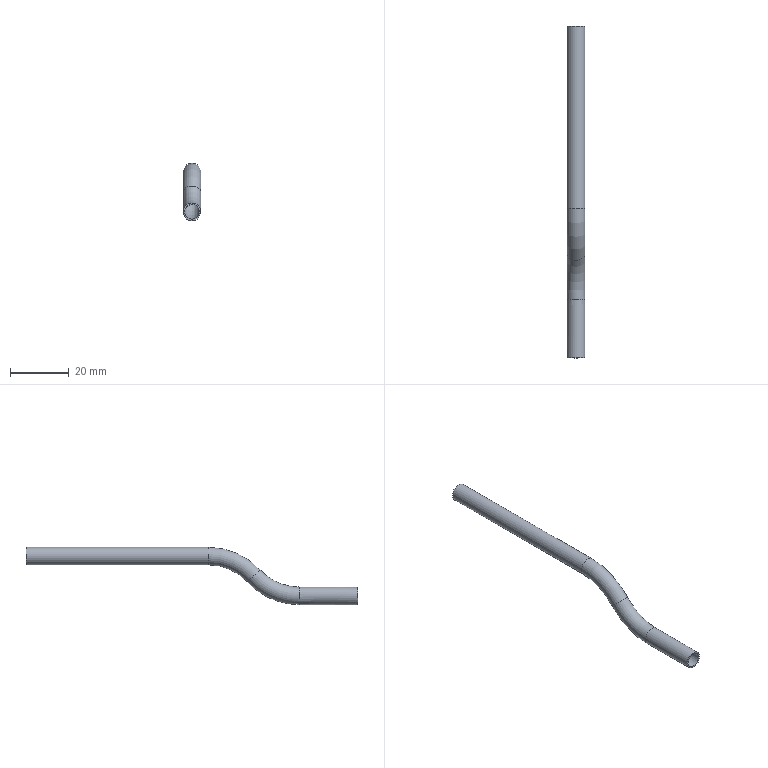Part | STEP file | 1-75.8 | 1 solid | 10 faces | box 6 x 112.85 x 19.5 mm | volume 1008 mm3 | cylinder 4 | torus 4 | plane 2 | commonest cylinder face diameters 5 x2 6 x2
STEP:
#1=CARTESIAN_POINT('',(0.,0.,0.));
#2=DIRECTION('',(0.,0.,1.));
#3=DIRECTION('',(1.,0.,0.));
#4=AXIS2_PLACEMENT_3D('',#1,#2,#3);
#5=CARTESIAN_POINT('',(3.,0.,0.));
#6=VERTEX_POINT('',#5);
#7=CARTESIAN_POINT('',(0.,0.,0.));
#8=DIRECTION('',(0.,-1.,0.));
#9=DIRECTION('',(1.,0.,0.));
#10=AXIS2_PLACEMENT_3D('',#7,#8,#9);
#11=CIRCLE('',#10,3.);
#12=CARTESIAN_POINT('',(0.,0.,0.));
#13=DIRECTION('',(0.,1.,0.));
#14=DIRECTION('',(1.,0.,0.));
#15=AXIS2_PLACEMENT_3D('',#12,#13,#14);
#16=CYLINDRICAL_SURFACE('',#15,3.);
#17=CARTESIAN_POINT('',(6.283,0.));
#18=DIRECTION('',(-1.,0.));
#19=VECTOR('',#18,1.);
#20=LINE('',#17,#19);
#21=(GEOMETRIC_REPRESENTATION_CONTEXT(2)PARAMETRIC_REPRESENTATION_CONTEXT()REPRESENTATION_CONTEXT('',''));
#22=DEFINITIONAL_REPRESENTATION('',(#20),#21);
#23=PCURVE('',#16,#22);
#24=CARTESIAN_POINT('',(0.,0.,0.));
#25=DIRECTION('',(0.,-1.,0.));
#26=DIRECTION('',(0.,0.,-1.));
#27=AXIS2_PLACEMENT_3D('',#24,#25,#26);
#28=PLANE('',#27);
#29=CARTESIAN_POINT('',(0.,0.));
#30=DIRECTION('',(0.,1.));
#31=AXIS2_PLACEMENT_2D('',#29,#30);
#32=CIRCLE('',#31,3.);
#33=(GEOMETRIC_REPRESENTATION_CONTEXT(2)PARAMETRIC_REPRESENTATION_CONTEXT()REPRESENTATION_CONTEXT('',''));
#34=DEFINITIONAL_REPRESENTATION('',(#32),#33);
#35=PCURVE('',#28,#34);
#36=SURFACE_CURVE('',#11,(#23,#35),.PCURVE_S1.);
#37=EDGE_CURVE('',#6,#6,#36,.T.);
#38=ORIENTED_EDGE('',*,*,#37,.F.);
#39=CARTESIAN_POINT('',(3.,20.,0.));
#40=VERTEX_POINT('',#39);
#41=CARTESIAN_POINT('',(3.,0.,0.));
#42=DIRECTION('',(0.,1.,0.));
#43=VECTOR('',#42,1.);
#44=LINE('',#41,#43);
#45=CARTESIAN_POINT('',(6.283,0.));
#46=DIRECTION('',(0.,1.));
#47=VECTOR('',#46,1.);
#48=LINE('',#45,#47);
#49=(GEOMETRIC_REPRESENTATION_CONTEXT(2)PARAMETRIC_REPRESENTATION_CONTEXT()REPRESENTATION_CONTEXT('',''));
#50=DEFINITIONAL_REPRESENTATION('',(#48),#49);
#51=PCURVE('',#16,#50);
#52=CARTESIAN_POINT('',(0.,0.));
#53=DIRECTION('',(0.,1.));
#54=VECTOR('',#53,1.);
#55=LINE('',#52,#54);
#56=(GEOMETRIC_REPRESENTATION_CONTEXT(2)PARAMETRIC_REPRESENTATION_CONTEXT()REPRESENTATION_CONTEXT('',''));
#57=DEFINITIONAL_REPRESENTATION('',(#55),#56);
#58=PCURVE('',#16,#57);
#59=SEAM_CURVE('',#44,(#51,#58),.PCURVE_S1.);
#60=EDGE_CURVE('',#6,#40,#59,.T.);
#61=ORIENTED_EDGE('',*,*,#60,.T.);
#62=CARTESIAN_POINT('',(0.,20.,-3.));
#63=VERTEX_POINT('',#62);
#64=CARTESIAN_POINT('',(0.,20.,0.));
#65=DIRECTION('',(0.,1.,0.));
#66=DIRECTION('',(0.,0.,-1.));
#67=AXIS2_PLACEMENT_3D('',#64,#65,#66);
#68=CIRCLE('',#67,3.);
#69=CARTESIAN_POINT('',(1.571,20.));
#70=DIRECTION('',(1.,0.));
#71=VECTOR('',#70,1.);
#72=LINE('',#69,#71);
#73=(GEOMETRIC_REPRESENTATION_CONTEXT(2)PARAMETRIC_REPRESENTATION_CONTEXT()REPRESENTATION_CONTEXT('',''));
#74=DEFINITIONAL_REPRESENTATION('',(#72),#73);
#75=PCURVE('',#16,#74);
#76=CARTESIAN_POINT('',(0.,20.,21.));
#77=DIRECTION('',(-1.,0.,0.));
#78=DIRECTION('',(0.,0.,-1.));
#79=AXIS2_PLACEMENT_3D('',#76,#77,#78);
#80=TOROIDAL_SURFACE('',#79,21.,3.);
#81=CARTESIAN_POINT('',(6.283,0.));
#82=DIRECTION('',(0.,1.));
#83=VECTOR('',#82,1.);
#84=LINE('',#81,#83);
#85=(GEOMETRIC_REPRESENTATION_CONTEXT(2)PARAMETRIC_REPRESENTATION_CONTEXT()REPRESENTATION_CONTEXT('',''));
#86=DEFINITIONAL_REPRESENTATION('',(#84),#85);
#87=PCURVE('',#80,#86);
#88=SURFACE_CURVE('',#68,(#75,#87),.PCURVE_S1.);
#89=EDGE_CURVE('',#63,#40,#88,.T.);
#90=ORIENTED_EDGE('',*,*,#89,.F.);
#91=CARTESIAN_POINT('',(0.,20.,0.));
#92=DIRECTION('',(0.,1.,0.));
#93=DIRECTION('',(1.,0.,0.));
#94=AXIS2_PLACEMENT_3D('',#91,#92,#93);
#95=CIRCLE('',#94,3.);
#96=CARTESIAN_POINT('',(0.,20.));
#97=DIRECTION('',(1.,0.));
#98=VECTOR('',#97,1.);
#99=LINE('',#96,#98);
#100=(GEOMETRIC_REPRESENTATION_CONTEXT(2)PARAMETRIC_REPRESENTATION_CONTEXT()REPRESENTATION_CONTEXT('',''));
#101=DEFINITIONAL_REPRESENTATION('',(#99),#100);
#102=PCURVE('',#16,#101);
#103=CARTESIAN_POINT('',(6.283,4.712));
#104=DIRECTION('',(0.,1.));
#105=VECTOR('',#104,1.);
#106=LINE('',#103,#105);
#107=(GEOMETRIC_REPRESENTATION_CONTEXT(2)PARAMETRIC_REPRESENTATION_CONTEXT()REPRESENTATION_CONTEXT('',''));
#108=DEFINITIONAL_REPRESENTATION('',(#106),#107);
#109=PCURVE('',#80,#108);
#110=SURFACE_CURVE('',#95,(#102,#109),.PCURVE_S1.);
#111=EDGE_CURVE('',#40,#63,#110,.T.);
#112=ORIENTED_EDGE('',*,*,#111,.F.);
#113=ORIENTED_EDGE('',*,*,#60,.F.);
#114=EDGE_LOOP('',(#38,#61,#90,#112,#113));
#115=FACE_BOUND('',#114,.T.);
#116=ADVANCED_FACE('',(#115),#16,.T.);
#117=ORIENTED_EDGE('',*,*,#89,.T.);
#118=ORIENTED_EDGE('',*,*,#111,.T.);
#119=CARTESIAN_POINT('',(0.,37.629,4.714));
#120=VERTEX_POINT('',#119);
#121=CARTESIAN_POINT('',(0.,20.,21.));
#122=DIRECTION('',(1.,0.,0.));
#123=DIRECTION('',(0.,0.,-1.));
#124=AXIS2_PLACEMENT_3D('',#121,#122,#123);
#125=CIRCLE('',#124,24.);
#126=CARTESIAN_POINT('',(6.283,6.283));
#127=DIRECTION('',(-1.,0.));
#128=VECTOR('',#127,1.);
#129=LINE('',#126,#128);
#130=(GEOMETRIC_REPRESENTATION_CONTEXT(2)PARAMETRIC_REPRESENTATION_CONTEXT()REPRESENTATION_CONTEXT('',''));
#131=DEFINITIONAL_REPRESENTATION('',(#129),#130);
#132=PCURVE('',#80,#131);
#133=CARTESIAN_POINT('',(6.283,0.));
#134=DIRECTION('',(-1.,0.));
#135=VECTOR('',#134,1.);
#136=LINE('',#133,#135);
#137=(GEOMETRIC_REPRESENTATION_CONTEXT(2)PARAMETRIC_REPRESENTATION_CONTEXT()REPRESENTATION_CONTEXT('',''));
#138=DEFINITIONAL_REPRESENTATION('',(#136),#137);
#139=PCURVE('',#80,#138);
#140=SEAM_CURVE('',#125,(#132,#139),.PCURVE_S1.);
#141=EDGE_CURVE('',#63,#120,#140,.T.);
#142=ORIENTED_EDGE('',*,*,#141,.T.);
#143=CARTESIAN_POINT('',(-3.,35.425,6.75));
#144=VERTEX_POINT('',#143);
#145=CARTESIAN_POINT('',(0.,35.425,6.75));
#146=DIRECTION('',(0.,-0.6786,-0.7345));
#147=DIRECTION('',(0.,0.7345,-0.6786));
#148=AXIS2_PLACEMENT_3D('',#145,#146,#147);
#149=CIRCLE('',#148,3.);
#150=CARTESIAN_POINT('',(5.458,6.283));
#151=DIRECTION('',(0.,-1.));
#152=VECTOR('',#151,1.);
#153=LINE('',#150,#152);
#154=(GEOMETRIC_REPRESENTATION_CONTEXT(2)PARAMETRIC_REPRESENTATION_CONTEXT()REPRESENTATION_CONTEXT('',''));
#155=DEFINITIONAL_REPRESENTATION('',(#153),#154);
#156=PCURVE('',#80,#155);
#157=CARTESIAN_POINT('',(0.,50.85,-7.5));
#158=DIRECTION('',(1.,0.,0.));
#159=DIRECTION('',(0.,-0.7345,0.6786));
#160=AXIS2_PLACEMENT_3D('',#157,#158,#159);
#161=TOROIDAL_SURFACE('',#160,21.,3.);
#162=CARTESIAN_POINT('',(6.283,3.142));
#163=DIRECTION('',(0.,-1.));
#164=VECTOR('',#163,1.);
#165=LINE('',#162,#164);
#166=(GEOMETRIC_REPRESENTATION_CONTEXT(2)PARAMETRIC_REPRESENTATION_CONTEXT()REPRESENTATION_CONTEXT('',''));
#167=DEFINITIONAL_REPRESENTATION('',(#165),#166);
#168=PCURVE('',#161,#167);
#169=SURFACE_CURVE('',#149,(#156,#168),.PCURVE_S1.);
#170=EDGE_CURVE('',#120,#144,#169,.T.);
#171=ORIENTED_EDGE('',*,*,#170,.T.);
#172=CARTESIAN_POINT('',(0.,35.425,6.75));
#173=DIRECTION('',(0.,-0.6786,-0.7345));
#174=DIRECTION('',(-1.,0.,0.));
#175=AXIS2_PLACEMENT_3D('',#172,#173,#174);
#176=CIRCLE('',#175,3.);
#177=CARTESIAN_POINT('',(5.458,1.571));
#178=DIRECTION('',(0.,-1.));
#179=VECTOR('',#178,1.);
#180=LINE('',#177,#179);
#181=(GEOMETRIC_REPRESENTATION_CONTEXT(2)PARAMETRIC_REPRESENTATION_CONTEXT()REPRESENTATION_CONTEXT('',''));
#182=DEFINITIONAL_REPRESENTATION('',(#180),#181);
#183=PCURVE('',#80,#182);
#184=CARTESIAN_POINT('',(6.283,4.712));
#185=DIRECTION('',(0.,-1.));
#186=VECTOR('',#185,1.);
#187=LINE('',#184,#186);
#188=(GEOMETRIC_REPRESENTATION_CONTEXT(2)PARAMETRIC_REPRESENTATION_CONTEXT()REPRESENTATION_CONTEXT('',''));
#189=DEFINITIONAL_REPRESENTATION('',(#187),#188);
#190=PCURVE('',#161,#189);
#191=SURFACE_CURVE('',#176,(#183,#190),.PCURVE_S1.);
#192=EDGE_CURVE('',#144,#120,#191,.T.);
#193=ORIENTED_EDGE('',*,*,#192,.T.);
#194=ORIENTED_EDGE('',*,*,#141,.F.);
#195=EDGE_LOOP('',(#117,#118,#142,#171,#193,#194));
#196=FACE_BOUND('',#195,.T.);
#197=ADVANCED_FACE('',(#196),#80,.T.);
#198=ORIENTED_EDGE('',*,*,#170,.F.);
#199=ORIENTED_EDGE('',*,*,#192,.F.);
#200=CARTESIAN_POINT('',(-3.,50.85,13.5));
#201=VERTEX_POINT('',#200);
#202=CARTESIAN_POINT('',(-3.,50.85,-7.5));
#203=DIRECTION('',(-1.,0.,0.));
#204=DIRECTION('',(0.,-0.7345,0.6786));
#205=AXIS2_PLACEMENT_3D('',#202,#203,#204);
#206=CIRCLE('',#205,21.);
#207=CARTESIAN_POINT('',(6.283,4.712));
#208=DIRECTION('',(-1.,0.));
#209=VECTOR('',#208,1.);
#210=LINE('',#207,#209);
#211=(GEOMETRIC_REPRESENTATION_CONTEXT(2)PARAMETRIC_REPRESENTATION_CONTEXT()REPRESENTATION_CONTEXT('',''));
#212=DEFINITIONAL_REPRESENTATION('',(#210),#211);
#213=PCURVE('',#161,#212);
#214=CARTESIAN_POINT('',(6.283,-1.571));
#215=DIRECTION('',(-1.,0.));
#216=VECTOR('',#215,1.);
#217=LINE('',#214,#216);
#218=(GEOMETRIC_REPRESENTATION_CONTEXT(2)PARAMETRIC_REPRESENTATION_CONTEXT()REPRESENTATION_CONTEXT('',''));
#219=DEFINITIONAL_REPRESENTATION('',(#217),#218);
#220=PCURVE('',#161,#219);
#221=SEAM_CURVE('',#206,(#213,#220),.PCURVE_S1.);
#222=EDGE_CURVE('',#144,#201,#221,.T.);
#223=ORIENTED_EDGE('',*,*,#222,.T.);
#224=CARTESIAN_POINT('',(3.,50.85,13.5));
#225=VERTEX_POINT('',#224);
#226=CARTESIAN_POINT('',(0.,50.85,13.5));
#227=DIRECTION('',(0.,-1.,0.));
#228=DIRECTION('',(-1.,0.,0.));
#229=AXIS2_PLACEMENT_3D('',#226,#227,#228);
#230=CIRCLE('',#229,3.);
#231=CARTESIAN_POINT('',(5.458,4.712));
#232=DIRECTION('',(0.,-1.));
#233=VECTOR('',#232,1.);
#234=LINE('',#231,#233);
#235=(GEOMETRIC_REPRESENTATION_CONTEXT(2)PARAMETRIC_REPRESENTATION_CONTEXT()REPRESENTATION_CONTEXT('',''));
#236=DEFINITIONAL_REPRESENTATION('',(#234),#235);
#237=PCURVE('',#161,#236);
#238=CARTESIAN_POINT('',(0.,50.85,13.5));
#239=DIRECTION('',(0.,1.,0.));
#240=DIRECTION('',(1.,0.,0.));
#241=AXIS2_PLACEMENT_3D('',#238,#239,#240);
#242=CYLINDRICAL_SURFACE('',#241,3.);
#243=CARTESIAN_POINT('',(3.142,0.));
#244=DIRECTION('',(-1.,0.));
#245=VECTOR('',#244,1.);
#246=LINE('',#243,#245);
#247=(GEOMETRIC_REPRESENTATION_CONTEXT(2)PARAMETRIC_REPRESENTATION_CONTEXT()REPRESENTATION_CONTEXT('',''));
#248=DEFINITIONAL_REPRESENTATION('',(#246),#247);
#249=PCURVE('',#242,#248);
#250=SURFACE_CURVE('',#230,(#237,#249),.PCURVE_S1.);
#251=EDGE_CURVE('',#201,#225,#250,.T.);
#252=ORIENTED_EDGE('',*,*,#251,.T.);
#253=CARTESIAN_POINT('',(0.,50.85,13.5));
#254=DIRECTION('',(0.,-1.,0.));
#255=DIRECTION('',(1.,0.,0.));
#256=AXIS2_PLACEMENT_3D('',#253,#254,#255);
#257=CIRCLE('',#256,3.);
#258=CARTESIAN_POINT('',(5.458,1.571));
#259=DIRECTION('',(0.,-1.));
#260=VECTOR('',#259,1.);
#261=LINE('',#258,#260);
#262=(GEOMETRIC_REPRESENTATION_CONTEXT(2)PARAMETRIC_REPRESENTATION_CONTEXT()REPRESENTATION_CONTEXT('',''));
#263=DEFINITIONAL_REPRESENTATION('',(#261),#262);
#264=PCURVE('',#161,#263);
#265=CARTESIAN_POINT('',(6.283,0.));
#266=DIRECTION('',(-1.,0.));
#267=VECTOR('',#266,1.);
#268=LINE('',#265,#267);
#269=(GEOMETRIC_REPRESENTATION_CONTEXT(2)PARAMETRIC_REPRESENTATION_CONTEXT()REPRESENTATION_CONTEXT('',''));
#270=DEFINITIONAL_REPRESENTATION('',(#268),#269);
#271=PCURVE('',#242,#270);
#272=SURFACE_CURVE('',#257,(#264,#271),.PCURVE_S1.);
#273=EDGE_CURVE('',#225,#201,#272,.T.);
#274=ORIENTED_EDGE('',*,*,#273,.T.);
#275=ORIENTED_EDGE('',*,*,#222,.F.);
#276=EDGE_LOOP('',(#198,#199,#223,#252,#274,#275));
#277=FACE_BOUND('',#276,.T.);
#278=ADVANCED_FACE('',(#277),#161,.T.);
#279=ORIENTED_EDGE('',*,*,#251,.F.);
#280=ORIENTED_EDGE('',*,*,#273,.F.);
#281=CARTESIAN_POINT('',(3.,112.85,13.5));
#282=VERTEX_POINT('',#281);
#283=CARTESIAN_POINT('',(3.,50.85,13.5));
#284=DIRECTION('',(0.,1.,0.));
#285=VECTOR('',#284,1.);
#286=LINE('',#283,#285);
#287=CARTESIAN_POINT('',(6.283,0.));
#288=DIRECTION('',(0.,1.));
#289=VECTOR('',#288,1.);
#290=LINE('',#287,#289);
#291=(GEOMETRIC_REPRESENTATION_CONTEXT(2)PARAMETRIC_REPRESENTATION_CONTEXT()REPRESENTATION_CONTEXT('',''));
#292=DEFINITIONAL_REPRESENTATION('',(#290),#291);
#293=PCURVE('',#242,#292);
#294=CARTESIAN_POINT('',(0.,0.));
#295=DIRECTION('',(0.,1.));
#296=VECTOR('',#295,1.);
#297=LINE('',#294,#296);
#298=(GEOMETRIC_REPRESENTATION_CONTEXT(2)PARAMETRIC_REPRESENTATION_CONTEXT()REPRESENTATION_CONTEXT('',''));
#299=DEFINITIONAL_REPRESENTATION('',(#297),#298);
#300=PCURVE('',#242,#299);
#301=SEAM_CURVE('',#286,(#293,#300),.PCURVE_S1.);
#302=EDGE_CURVE('',#225,#282,#301,.T.);
#303=ORIENTED_EDGE('',*,*,#302,.T.);
#304=CARTESIAN_POINT('',(0.,112.85,13.5));
#305=DIRECTION('',(0.,1.,0.));
#306=DIRECTION('',(1.,0.,0.));
#307=AXIS2_PLACEMENT_3D('',#304,#305,#306);
#308=CIRCLE('',#307,3.);
#309=CARTESIAN_POINT('',(0.,62.));
#310=DIRECTION('',(1.,0.));
#311=VECTOR('',#310,1.);
#312=LINE('',#309,#311);
#313=(GEOMETRIC_REPRESENTATION_CONTEXT(2)PARAMETRIC_REPRESENTATION_CONTEXT()REPRESENTATION_CONTEXT('',''));
#314=DEFINITIONAL_REPRESENTATION('',(#312),#313);
#315=PCURVE('',#242,#314);
#316=CARTESIAN_POINT('',(0.,112.85,13.5));
#317=DIRECTION('',(0.,1.,0.));
#318=DIRECTION('',(0.,0.,1.));
#319=AXIS2_PLACEMENT_3D('',#316,#317,#318);
#320=PLANE('',#319);
#321=CARTESIAN_POINT('',(0.,0.));
#322=DIRECTION('',(0.,1.));
#323=AXIS2_PLACEMENT_2D('',#321,#322);
#324=CIRCLE('',#323,3.);
#325=(GEOMETRIC_REPRESENTATION_CONTEXT(2)PARAMETRIC_REPRESENTATION_CONTEXT()REPRESENTATION_CONTEXT('',''));
#326=DEFINITIONAL_REPRESENTATION('',(#324),#325);
#327=PCURVE('',#320,#326);
#328=SURFACE_CURVE('',#308,(#315,#327),.PCURVE_S1.);
#329=EDGE_CURVE('',#282,#282,#328,.T.);
#330=ORIENTED_EDGE('',*,*,#329,.F.);
#331=ORIENTED_EDGE('',*,*,#302,.F.);
#332=EDGE_LOOP('',(#279,#280,#303,#330,#331));
#333=FACE_BOUND('',#332,.T.);
#334=ADVANCED_FACE('',(#333),#242,.T.);
#335=ORIENTED_EDGE('',*,*,#37,.T.);
#336=EDGE_LOOP('',(#335));
#337=FACE_BOUND('',#336,.T.);
#338=CARTESIAN_POINT('',(2.5,0.,0.));
#339=VERTEX_POINT('',#338);
#340=CARTESIAN_POINT('',(0.,0.,0.));
#341=DIRECTION('',(0.,-1.,0.));
#342=DIRECTION('',(1.,0.,0.));
#343=AXIS2_PLACEMENT_3D('',#340,#341,#342);
#344=CIRCLE('',#343,2.5);
#345=CARTESIAN_POINT('',(0.,0.));
#346=DIRECTION('',(0.,1.));
#347=AXIS2_PLACEMENT_2D('',#345,#346);
#348=CIRCLE('',#347,2.5);
#349=(GEOMETRIC_REPRESENTATION_CONTEXT(2)PARAMETRIC_REPRESENTATION_CONTEXT()REPRESENTATION_CONTEXT('',''));
#350=DEFINITIONAL_REPRESENTATION('',(#348),#349);
#351=PCURVE('',#28,#350);
#352=CARTESIAN_POINT('',(0.,0.,0.));
#353=DIRECTION('',(0.,1.,0.));
#354=DIRECTION('',(1.,0.,0.));
#355=AXIS2_PLACEMENT_3D('',#352,#353,#354);
#356=CYLINDRICAL_SURFACE('',#355,2.5);
#357=CARTESIAN_POINT('',(6.283,0.));
#358=DIRECTION('',(-1.,0.));
#359=VECTOR('',#358,1.);
#360=LINE('',#357,#359);
#361=(GEOMETRIC_REPRESENTATION_CONTEXT(2)PARAMETRIC_REPRESENTATION_CONTEXT()REPRESENTATION_CONTEXT('',''));
#362=DEFINITIONAL_REPRESENTATION('',(#360),#361);
#363=PCURVE('',#356,#362);
#364=SURFACE_CURVE('',#344,(#351,#363),.PCURVE_S1.);
#365=EDGE_CURVE('',#339,#339,#364,.T.);
#366=ORIENTED_EDGE('',*,*,#365,.F.);
#367=EDGE_LOOP('',(#366));
#368=FACE_BOUND('',#367,.T.);
#369=ADVANCED_FACE('',(#337,#368),#28,.T.);
#370=ORIENTED_EDGE('',*,*,#329,.T.);
#371=EDGE_LOOP('',(#370));
#372=FACE_BOUND('',#371,.T.);
#373=CARTESIAN_POINT('',(2.5,112.85,13.5));
#374=VERTEX_POINT('',#373);
#375=CARTESIAN_POINT('',(0.,112.85,13.5));
#376=DIRECTION('',(0.,1.,0.));
#377=DIRECTION('',(1.,0.,0.));
#378=AXIS2_PLACEMENT_3D('',#375,#376,#377);
#379=CIRCLE('',#378,2.5);
#380=CARTESIAN_POINT('',(0.,0.));
#381=DIRECTION('',(0.,1.));
#382=AXIS2_PLACEMENT_2D('',#380,#381);
#383=CIRCLE('',#382,2.5);
#384=(GEOMETRIC_REPRESENTATION_CONTEXT(2)PARAMETRIC_REPRESENTATION_CONTEXT()REPRESENTATION_CONTEXT('',''));
#385=DEFINITIONAL_REPRESENTATION('',(#383),#384);
#386=PCURVE('',#320,#385);
#387=CARTESIAN_POINT('',(0.,50.85,13.5));
#388=DIRECTION('',(0.,1.,0.));
#389=DIRECTION('',(1.,0.,0.));
#390=AXIS2_PLACEMENT_3D('',#387,#388,#389);
#391=CYLINDRICAL_SURFACE('',#390,2.5);
#392=CARTESIAN_POINT('',(0.,62.));
#393=DIRECTION('',(1.,0.));
#394=VECTOR('',#393,1.);
#395=LINE('',#392,#394);
#396=(GEOMETRIC_REPRESENTATION_CONTEXT(2)PARAMETRIC_REPRESENTATION_CONTEXT()REPRESENTATION_CONTEXT('',''));
#397=DEFINITIONAL_REPRESENTATION('',(#395),#396);
#398=PCURVE('',#391,#397);
#399=SURFACE_CURVE('',#379,(#386,#398),.PCURVE_S1.);
#400=EDGE_CURVE('',#374,#374,#399,.T.);
#401=ORIENTED_EDGE('',*,*,#400,.F.);
#402=EDGE_LOOP('',(#401));
#403=FACE_BOUND('',#402,.T.);
#404=ADVANCED_FACE('',(#372,#403),#320,.T.);
#405=ORIENTED_EDGE('',*,*,#365,.F.);
#406=CARTESIAN_POINT('',(2.5,20.,0.));
#407=VERTEX_POINT('',#406);
#408=CARTESIAN_POINT('',(2.5,0.,0.));
#409=DIRECTION('',(0.,1.,0.));
#410=VECTOR('',#409,1.);
#411=LINE('',#408,#410);
#412=CARTESIAN_POINT('',(6.283,0.));
#413=DIRECTION('',(0.,1.));
#414=VECTOR('',#413,1.);
#415=LINE('',#412,#414);
#416=(GEOMETRIC_REPRESENTATION_CONTEXT(2)PARAMETRIC_REPRESENTATION_CONTEXT()REPRESENTATION_CONTEXT('',''));
#417=DEFINITIONAL_REPRESENTATION('',(#415),#416);
#418=PCURVE('',#356,#417);
#419=CARTESIAN_POINT('',(0.,0.));
#420=DIRECTION('',(0.,1.));
#421=VECTOR('',#420,1.);
#422=LINE('',#419,#421);
#423=(GEOMETRIC_REPRESENTATION_CONTEXT(2)PARAMETRIC_REPRESENTATION_CONTEXT()REPRESENTATION_CONTEXT('',''));
#424=DEFINITIONAL_REPRESENTATION('',(#422),#423);
#425=PCURVE('',#356,#424);
#426=SEAM_CURVE('',#411,(#418,#425),.PCURVE_S1.);
#427=EDGE_CURVE('',#339,#407,#426,.T.);
#428=ORIENTED_EDGE('',*,*,#427,.T.);
#429=CARTESIAN_POINT('',(0.,20.,-2.5));
#430=VERTEX_POINT('',#429);
#431=CARTESIAN_POINT('',(0.,20.,0.));
#432=DIRECTION('',(0.,1.,0.));
#433=DIRECTION('',(0.,0.,-1.));
#434=AXIS2_PLACEMENT_3D('',#431,#432,#433);
#435=CIRCLE('',#434,2.5);
#436=CARTESIAN_POINT('',(1.571,20.));
#437=DIRECTION('',(1.,0.));
#438=VECTOR('',#437,1.);
#439=LINE('',#436,#438);
#440=(GEOMETRIC_REPRESENTATION_CONTEXT(2)PARAMETRIC_REPRESENTATION_CONTEXT()REPRESENTATION_CONTEXT('',''));
#441=DEFINITIONAL_REPRESENTATION('',(#439),#440);
#442=PCURVE('',#356,#441);
#443=CARTESIAN_POINT('',(0.,20.,21.));
#444=DIRECTION('',(-1.,0.,0.));
#445=DIRECTION('',(0.,0.,-1.));
#446=AXIS2_PLACEMENT_3D('',#443,#444,#445);
#447=TOROIDAL_SURFACE('',#446,21.,2.5);
#448=CARTESIAN_POINT('',(6.283,0.));
#449=DIRECTION('',(0.,1.));
#450=VECTOR('',#449,1.);
#451=LINE('',#448,#450);
#452=(GEOMETRIC_REPRESENTATION_CONTEXT(2)PARAMETRIC_REPRESENTATION_CONTEXT()REPRESENTATION_CONTEXT('',''));
#453=DEFINITIONAL_REPRESENTATION('',(#451),#452);
#454=PCURVE('',#447,#453);
#455=SURFACE_CURVE('',#435,(#442,#454),.PCURVE_S1.);
#456=EDGE_CURVE('',#430,#407,#455,.T.);
#457=ORIENTED_EDGE('',*,*,#456,.F.);
#458=CARTESIAN_POINT('',(0.,20.,0.));
#459=DIRECTION('',(0.,1.,0.));
#460=DIRECTION('',(1.,0.,0.));
#461=AXIS2_PLACEMENT_3D('',#458,#459,#460);
#462=CIRCLE('',#461,2.5);
#463=CARTESIAN_POINT('',(0.,20.));
#464=DIRECTION('',(1.,0.));
#465=VECTOR('',#464,1.);
#466=LINE('',#463,#465);
#467=(GEOMETRIC_REPRESENTATION_CONTEXT(2)PARAMETRIC_REPRESENTATION_CONTEXT()REPRESENTATION_CONTEXT('',''));
#468=DEFINITIONAL_REPRESENTATION('',(#466),#467);
#469=PCURVE('',#356,#468);
#470=CARTESIAN_POINT('',(6.283,4.712));
#471=DIRECTION('',(0.,1.));
#472=VECTOR('',#471,1.);
#473=LINE('',#470,#472);
#474=(GEOMETRIC_REPRESENTATION_CONTEXT(2)PARAMETRIC_REPRESENTATION_CONTEXT()REPRESENTATION_CONTEXT('',''));
#475=DEFINITIONAL_REPRESENTATION('',(#473),#474);
#476=PCURVE('',#447,#475);
#477=SURFACE_CURVE('',#462,(#469,#476),.PCURVE_S1.);
#478=EDGE_CURVE('',#407,#430,#477,.T.);
#479=ORIENTED_EDGE('',*,*,#478,.F.);
#480=ORIENTED_EDGE('',*,*,#427,.F.);
#481=EDGE_LOOP('',(#405,#428,#457,#479,#480));
#482=FACE_BOUND('',#481,.F.);
#483=ADVANCED_FACE('',(#482),#356,.F.);
#484=ORIENTED_EDGE('',*,*,#456,.T.);
#485=ORIENTED_EDGE('',*,*,#478,.T.);
#486=CARTESIAN_POINT('',(0.,37.262,5.054));
#487=VERTEX_POINT('',#486);
#488=CARTESIAN_POINT('',(0.,20.,21.));
#489=DIRECTION('',(1.,0.,0.));
#490=DIRECTION('',(0.,0.,-1.));
#491=AXIS2_PLACEMENT_3D('',#488,#489,#490);
#492=CIRCLE('',#491,23.5);
#493=CARTESIAN_POINT('',(6.283,6.283));
#494=DIRECTION('',(-1.,0.));
#495=VECTOR('',#494,1.);
#496=LINE('',#493,#495);
#497=(GEOMETRIC_REPRESENTATION_CONTEXT(2)PARAMETRIC_REPRESENTATION_CONTEXT()REPRESENTATION_CONTEXT('',''));
#498=DEFINITIONAL_REPRESENTATION('',(#496),#497);
#499=PCURVE('',#447,#498);
#500=CARTESIAN_POINT('',(6.283,0.));
#501=DIRECTION('',(-1.,0.));
#502=VECTOR('',#501,1.);
#503=LINE('',#500,#502);
#504=(GEOMETRIC_REPRESENTATION_CONTEXT(2)PARAMETRIC_REPRESENTATION_CONTEXT()REPRESENTATION_CONTEXT('',''));
#505=DEFINITIONAL_REPRESENTATION('',(#503),#504);
#506=PCURVE('',#447,#505);
#507=SEAM_CURVE('',#492,(#499,#506),.PCURVE_S1.);
#508=EDGE_CURVE('',#430,#487,#507,.T.);
#509=ORIENTED_EDGE('',*,*,#508,.T.);
#510=CARTESIAN_POINT('',(-2.5,35.425,6.75));
#511=VERTEX_POINT('',#510);
#512=CARTESIAN_POINT('',(0.,35.425,6.75));
#513=DIRECTION('',(0.,-0.6786,-0.7345));
#514=DIRECTION('',(0.,0.7345,-0.6786));
#515=AXIS2_PLACEMENT_3D('',#512,#513,#514);
#516=CIRCLE('',#515,2.5);
#517=CARTESIAN_POINT('',(5.458,6.283));
#518=DIRECTION('',(0.,-1.));
#519=VECTOR('',#518,1.);
#520=LINE('',#517,#519);
#521=(GEOMETRIC_REPRESENTATION_CONTEXT(2)PARAMETRIC_REPRESENTATION_CONTEXT()REPRESENTATION_CONTEXT('',''));
#522=DEFINITIONAL_REPRESENTATION('',(#520),#521);
#523=PCURVE('',#447,#522);
#524=CARTESIAN_POINT('',(0.,50.85,-7.5));
#525=DIRECTION('',(1.,0.,0.));
#526=DIRECTION('',(0.,-0.7345,0.6786));
#527=AXIS2_PLACEMENT_3D('',#524,#525,#526);
#528=TOROIDAL_SURFACE('',#527,21.,2.5);
#529=CARTESIAN_POINT('',(6.283,3.142));
#530=DIRECTION('',(0.,-1.));
#531=VECTOR('',#530,1.);
#532=LINE('',#529,#531);
#533=(GEOMETRIC_REPRESENTATION_CONTEXT(2)PARAMETRIC_REPRESENTATION_CONTEXT()REPRESENTATION_CONTEXT('',''));
#534=DEFINITIONAL_REPRESENTATION('',(#532),#533);
#535=PCURVE('',#528,#534);
#536=SURFACE_CURVE('',#516,(#523,#535),.PCURVE_S1.);
#537=EDGE_CURVE('',#487,#511,#536,.T.);
#538=ORIENTED_EDGE('',*,*,#537,.T.);
#539=CARTESIAN_POINT('',(0.,35.425,6.75));
#540=DIRECTION('',(0.,-0.6786,-0.7345));
#541=DIRECTION('',(-1.,0.,0.));
#542=AXIS2_PLACEMENT_3D('',#539,#540,#541);
#543=CIRCLE('',#542,2.5);
#544=CARTESIAN_POINT('',(5.458,1.571));
#545=DIRECTION('',(0.,-1.));
#546=VECTOR('',#545,1.);
#547=LINE('',#544,#546);
#548=(GEOMETRIC_REPRESENTATION_CONTEXT(2)PARAMETRIC_REPRESENTATION_CONTEXT()REPRESENTATION_CONTEXT('',''));
#549=DEFINITIONAL_REPRESENTATION('',(#547),#548);
#550=PCURVE('',#447,#549);
#551=CARTESIAN_POINT('',(6.283,4.712));
#552=DIRECTION('',(0.,-1.));
#553=VECTOR('',#552,1.);
#554=LINE('',#551,#553);
#555=(GEOMETRIC_REPRESENTATION_CONTEXT(2)PARAMETRIC_REPRESENTATION_CONTEXT()REPRESENTATION_CONTEXT('',''));
#556=DEFINITIONAL_REPRESENTATION('',(#554),#555);
#557=PCURVE('',#528,#556);
#558=SURFACE_CURVE('',#543,(#550,#557),.PCURVE_S1.);
#559=EDGE_CURVE('',#511,#487,#558,.T.);
#560=ORIENTED_EDGE('',*,*,#559,.T.);
#561=ORIENTED_EDGE('',*,*,#508,.F.);
#562=EDGE_LOOP('',(#484,#485,#509,#538,#560,#561));
#563=FACE_BOUND('',#562,.F.);
#564=ADVANCED_FACE('',(#563),#447,.F.);
#565=ORIENTED_EDGE('',*,*,#537,.F.);
#566=ORIENTED_EDGE('',*,*,#559,.F.);
#567=CARTESIAN_POINT('',(-2.5,50.85,13.5));
#568=VERTEX_POINT('',#567);
#569=CARTESIAN_POINT('',(-2.5,50.85,-7.5));
#570=DIRECTION('',(-1.,0.,0.));
#571=DIRECTION('',(0.,-0.7345,0.6786));
#572=AXIS2_PLACEMENT_3D('',#569,#570,#571);
#573=CIRCLE('',#572,21.);
#574=CARTESIAN_POINT('',(6.283,4.712));
#575=DIRECTION('',(-1.,0.));
#576=VECTOR('',#575,1.);
#577=LINE('',#574,#576);
#578=(GEOMETRIC_REPRESENTATION_CONTEXT(2)PARAMETRIC_REPRESENTATION_CONTEXT()REPRESENTATION_CONTEXT('',''));
#579=DEFINITIONAL_REPRESENTATION('',(#577),#578);
#580=PCURVE('',#528,#579);
#581=CARTESIAN_POINT('',(6.283,-1.571));
#582=DIRECTION('',(-1.,0.));
#583=VECTOR('',#582,1.);
#584=LINE('',#581,#583);
#585=(GEOMETRIC_REPRESENTATION_CONTEXT(2)PARAMETRIC_REPRESENTATION_CONTEXT()REPRESENTATION_CONTEXT('',''));
#586=DEFINITIONAL_REPRESENTATION('',(#584),#585);
#587=PCURVE('',#528,#586);
#588=SEAM_CURVE('',#573,(#580,#587),.PCURVE_S1.);
#589=EDGE_CURVE('',#511,#568,#588,.T.);
#590=ORIENTED_EDGE('',*,*,#589,.T.);
#591=CARTESIAN_POINT('',(2.5,50.85,13.5));
#592=VERTEX_POINT('',#591);
#593=CARTESIAN_POINT('',(0.,50.85,13.5));
#594=DIRECTION('',(0.,-1.,0.));
#595=DIRECTION('',(-1.,0.,0.));
#596=AXIS2_PLACEMENT_3D('',#593,#594,#595);
#597=CIRCLE('',#596,2.5);
#598=CARTESIAN_POINT('',(5.458,4.712));
#599=DIRECTION('',(0.,-1.));
#600=VECTOR('',#599,1.);
#601=LINE('',#598,#600);
#602=(GEOMETRIC_REPRESENTATION_CONTEXT(2)PARAMETRIC_REPRESENTATION_CONTEXT()REPRESENTATION_CONTEXT('',''));
#603=DEFINITIONAL_REPRESENTATION('',(#601),#602);
#604=PCURVE('',#528,#603);
#605=CARTESIAN_POINT('',(3.142,0.));
#606=DIRECTION('',(-1.,0.));
#607=VECTOR('',#606,1.);
#608=LINE('',#605,#607);
#609=(GEOMETRIC_REPRESENTATION_CONTEXT(2)PARAMETRIC_REPRESENTATION_CONTEXT()REPRESENTATION_CONTEXT('',''));
#610=DEFINITIONAL_REPRESENTATION('',(#608),#609);
#611=PCURVE('',#391,#610);
#612=SURFACE_CURVE('',#597,(#604,#611),.PCURVE_S1.);
#613=EDGE_CURVE('',#568,#592,#612,.T.);
#614=ORIENTED_EDGE('',*,*,#613,.T.);
#615=CARTESIAN_POINT('',(0.,50.85,13.5));
#616=DIRECTION('',(0.,-1.,0.));
#617=DIRECTION('',(1.,0.,0.));
#618=AXIS2_PLACEMENT_3D('',#615,#616,#617);
#619=CIRCLE('',#618,2.5);
#620=CARTESIAN_POINT('',(5.458,1.571));
#621=DIRECTION('',(0.,-1.));
#622=VECTOR('',#621,1.);
#623=LINE('',#620,#622);
#624=(GEOMETRIC_REPRESENTATION_CONTEXT(2)PARAMETRIC_REPRESENTATION_CONTEXT()REPRESENTATION_CONTEXT('',''));
#625=DEFINITIONAL_REPRESENTATION('',(#623),#624);
#626=PCURVE('',#528,#625);
#627=CARTESIAN_POINT('',(6.283,0.));
#628=DIRECTION('',(-1.,0.));
#629=VECTOR('',#628,1.);
#630=LINE('',#627,#629);
#631=(GEOMETRIC_REPRESENTATION_CONTEXT(2)PARAMETRIC_REPRESENTATION_CONTEXT()REPRESENTATION_CONTEXT('',''));
#632=DEFINITIONAL_REPRESENTATION('',(#630),#631);
#633=PCURVE('',#391,#632);
#634=SURFACE_CURVE('',#619,(#626,#633),.PCURVE_S1.);
#635=EDGE_CURVE('',#592,#568,#634,.T.);
#636=ORIENTED_EDGE('',*,*,#635,.T.);
#637=ORIENTED_EDGE('',*,*,#589,.F.);
#638=EDGE_LOOP('',(#565,#566,#590,#614,#636,#637));
#639=FACE_BOUND('',#638,.F.);
#640=ADVANCED_FACE('',(#639),#528,.F.);
#641=ORIENTED_EDGE('',*,*,#613,.F.);
#642=ORIENTED_EDGE('',*,*,#635,.F.);
#643=CARTESIAN_POINT('',(2.5,50.85,13.5));
#644=DIRECTION('',(0.,1.,0.));
#645=VECTOR('',#644,1.);
#646=LINE('',#643,#645);
#647=CARTESIAN_POINT('',(6.283,0.));
#648=DIRECTION('',(0.,1.));
#649=VECTOR('',#648,1.);
#650=LINE('',#647,#649);
#651=(GEOMETRIC_REPRESENTATION_CONTEXT(2)PARAMETRIC_REPRESENTATION_CONTEXT()REPRESENTATION_CONTEXT('',''));
#652=DEFINITIONAL_REPRESENTATION('',(#650),#651);
#653=PCURVE('',#391,#652);
#654=CARTESIAN_POINT('',(0.,0.));
#655=DIRECTION('',(0.,1.));
#656=VECTOR('',#655,1.);
#657=LINE('',#654,#656);
#658=(GEOMETRIC_REPRESENTATION_CONTEXT(2)PARAMETRIC_REPRESENTATION_CONTEXT()REPRESENTATION_CONTEXT('',''));
#659=DEFINITIONAL_REPRESENTATION('',(#657),#658);
#660=PCURVE('',#391,#659);
#661=SEAM_CURVE('',#646,(#653,#660),.PCURVE_S1.);
#662=EDGE_CURVE('',#592,#374,#661,.T.);
#663=ORIENTED_EDGE('',*,*,#662,.T.);
#664=ORIENTED_EDGE('',*,*,#400,.F.);
#665=ORIENTED_EDGE('',*,*,#662,.F.);
#666=EDGE_LOOP('',(#641,#642,#663,#664,#665));
#667=FACE_BOUND('',#666,.F.);
#668=ADVANCED_FACE('',(#667),#391,.F.);
#669=CLOSED_SHELL('',(#116,#197,#278,#334,#369,#404,#483,#564,#640,#668));
#670=MANIFOLD_SOLID_BREP('',#669);
#671=(LENGTH_UNIT()NAMED_UNIT(*)SI_UNIT(.MILLI.,.METRE.));
#672=UNCERTAINTY_MEASURE_WITH_UNIT(LENGTH_MEASURE(0.0000001),#671,'','');
#673=(NAMED_UNIT(*)PLANE_ANGLE_UNIT()SI_UNIT($,.RADIAN.));
#674=(NAMED_UNIT(*)SI_UNIT($,.STERADIAN.)SOLID_ANGLE_UNIT());
#675=(GEOMETRIC_REPRESENTATION_CONTEXT(3)GLOBAL_UNCERTAINTY_ASSIGNED_CONTEXT((#672))GLOBAL_UNIT_ASSIGNED_CONTEXT((#671,#673,#674))REPRESENTATION_CONTEXT('',''));
#676=ADVANCED_BREP_SHAPE_REPRESENTATION('',(#4,#670),#675);